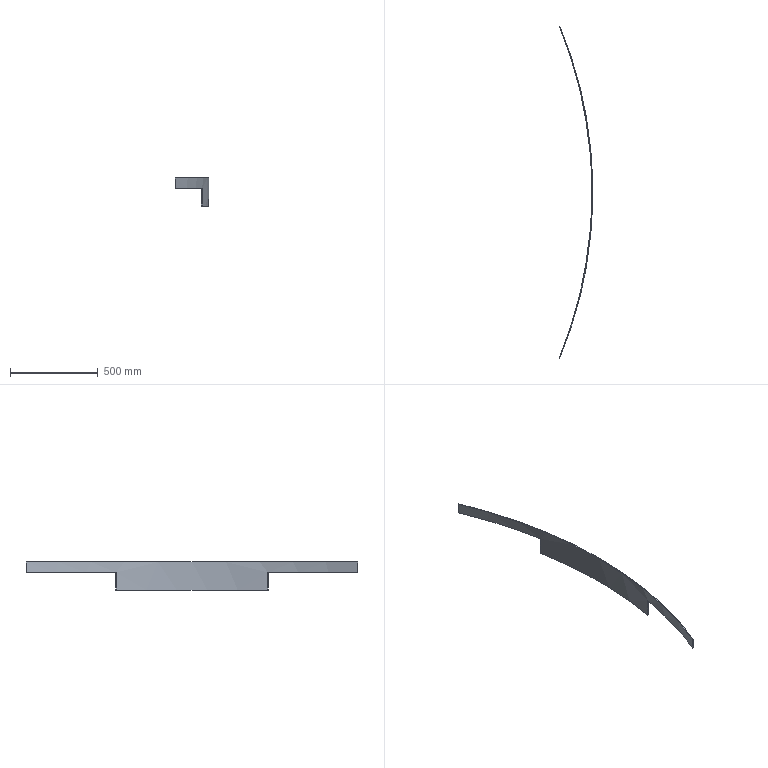Part | STEP file | 24B-Side baffle 2 | 1 solid | 10 faces | box 190.691 x 1891 x 160 mm | volume 813219 mm3 | plane 8 | cylinder 2 | commonest cylinder face diameters 4960 x1 4968 x1
STEP:
#1=CARTESIAN_POINT('',(0.,0.,0.));
#2=DIRECTION('',(0.,0.,1.));
#3=DIRECTION('',(1.,0.,0.));
#4=AXIS2_PLACEMENT_3D('',#1,#2,#3);
#5=CARTESIAN_POINT('',(2445.947,-433.125,100.));
#6=VERTEX_POINT('',#5);
#7=CARTESIAN_POINT('',(2442.009,-432.428,100.));
#8=VERTEX_POINT('',#7);
#9=CARTESIAN_POINT('',(2442.009,-432.428,100.));
#10=DIRECTION('',(-0.9847,0.1744,0.));
#11=VECTOR('',#10,1.);
#12=LINE('',#9,#11);
#13=CARTESIAN_POINT('',(0.,0.,100.));
#14=DIRECTION('',(0.,0.,1.));
#15=DIRECTION('',(1.,0.,0.));
#16=AXIS2_PLACEMENT_3D('',#13,#14,#15);
#17=PLANE('',#16);
#18=CARTESIAN_POINT('',(2442.009,-432.428));
#19=DIRECTION('',(-0.9847,0.1744));
#20=VECTOR('',#19,1.);
#21=LINE('',#18,#20);
#22=(GEOMETRIC_REPRESENTATION_CONTEXT(2)PARAMETRIC_REPRESENTATION_CONTEXT()REPRESENTATION_CONTEXT('',''));
#23=DEFINITIONAL_REPRESENTATION('',(#21),#22);
#24=PCURVE('',#17,#23);
#25=CARTESIAN_POINT('',(2442.009,-432.428,50.));
#26=DIRECTION('',(0.1744,0.9847,0.));
#27=DIRECTION('',(0.,0.,1.));
#28=AXIS2_PLACEMENT_3D('',#25,#26,#27);
#29=PLANE('',#28);
#30=CARTESIAN_POINT('',(50.,0.));
#31=DIRECTION('',(0.,-1.));
#32=VECTOR('',#31,1.);
#33=LINE('',#30,#32);
#34=(GEOMETRIC_REPRESENTATION_CONTEXT(2)PARAMETRIC_REPRESENTATION_CONTEXT()REPRESENTATION_CONTEXT('',''));
#35=DEFINITIONAL_REPRESENTATION('',(#33),#34);
#36=PCURVE('',#29,#35);
#37=SURFACE_CURVE('',#12,(#24,#36),.PCURVE_S1.);
#38=EDGE_CURVE('',#6,#8,#37,.T.);
#39=ORIENTED_EDGE('',*,*,#38,.F.);
#40=CARTESIAN_POINT('',(2297.007,-945.523,100.));
#41=VERTEX_POINT('',#40);
#42=CARTESIAN_POINT('',(0.,0.,100.));
#43=DIRECTION('',(0.,0.,-1.));
#44=DIRECTION('',(-1.,0.,0.));
#45=AXIS2_PLACEMENT_3D('',#42,#43,#44);
#46=CIRCLE('',#45,2484.);
#47=CARTESIAN_POINT('',(-2484.,0.));
#48=CARTESIAN_POINT('',(-2484.,4302.414));
#49=CARTESIAN_POINT('',(1242.,2151.207));
#50=CARTESIAN_POINT('',(4968.,0.));
#51=CARTESIAN_POINT('',(1242.,-2151.207));
#52=CARTESIAN_POINT('',(-2484.,-4302.414));
#53=CARTESIAN_POINT('',(-2484.,0.));
#54=(BOUNDED_CURVE()B_SPLINE_CURVE(2,(#47,#48,#49,#50,#51,#52,#53),.UNSPECIFIED.,.T.,.F.)B_SPLINE_CURVE_WITH_KNOTS((1,2,2,2,2,1),(-2.094,0.,2.094,4.189,6.283,8.378),.UNSPECIFIED.)CURVE()GEOMETRIC_REPRESENTATION_ITEM()RATIONAL_B_SPLINE_CURVE((1.,0.5,1.,0.5,1.,0.5,1.))REPRESENTATION_ITEM(''));
#55=(GEOMETRIC_REPRESENTATION_CONTEXT(2)PARAMETRIC_REPRESENTATION_CONTEXT()REPRESENTATION_CONTEXT('',''));
#56=DEFINITIONAL_REPRESENTATION('',(#54),#55);
#57=PCURVE('',#17,#56);
#58=CARTESIAN_POINT('',(0.,0.,2077.812));
#59=DIRECTION('',(0.,0.,-1.));
#60=DIRECTION('',(-1.,0.,0.));
#61=AXIS2_PLACEMENT_3D('',#58,#59,#60);
#62=CYLINDRICAL_SURFACE('',#61,2484.);
#63=CARTESIAN_POINT('',(0.,1977.812));
#64=DIRECTION('',(1.,0.));
#65=VECTOR('',#64,1.);
#66=LINE('',#63,#65);
#67=(GEOMETRIC_REPRESENTATION_CONTEXT(2)PARAMETRIC_REPRESENTATION_CONTEXT()REPRESENTATION_CONTEXT('',''));
#68=DEFINITIONAL_REPRESENTATION('',(#66),#67);
#69=PCURVE('',#62,#68);
#70=SURFACE_CURVE('',#46,(#57,#69),.PCURVE_S1.);
#71=EDGE_CURVE('',#6,#41,#70,.T.);
#72=ORIENTED_EDGE('',*,*,#71,.T.);
#73=CARTESIAN_POINT('',(2293.309,-944.,100.));
#74=VERTEX_POINT('',#73);
#75=CARTESIAN_POINT('',(2293.309,-944.,100.));
#76=DIRECTION('',(-0.9247,0.3806,0.));
#77=VECTOR('',#76,1.);
#78=LINE('',#75,#77);
#79=CARTESIAN_POINT('',(2293.309,-944.));
#80=DIRECTION('',(-0.9247,0.3806));
#81=VECTOR('',#80,1.);
#82=LINE('',#79,#81);
#83=(GEOMETRIC_REPRESENTATION_CONTEXT(2)PARAMETRIC_REPRESENTATION_CONTEXT()REPRESENTATION_CONTEXT('',''));
#84=DEFINITIONAL_REPRESENTATION('',(#82),#83);
#85=PCURVE('',#17,#84);
#86=CARTESIAN_POINT('',(2293.309,-944.,130.));
#87=DIRECTION('',(0.3806,0.9247,0.));
#88=DIRECTION('',(0.,0.,1.));
#89=AXIS2_PLACEMENT_3D('',#86,#87,#88);
#90=PLANE('',#89);
#91=CARTESIAN_POINT('',(-30.,0.));
#92=DIRECTION('',(0.,-1.));
#93=VECTOR('',#92,1.);
#94=LINE('',#91,#93);
#95=(GEOMETRIC_REPRESENTATION_CONTEXT(2)PARAMETRIC_REPRESENTATION_CONTEXT()REPRESENTATION_CONTEXT('',''));
#96=DEFINITIONAL_REPRESENTATION('',(#94),#95);
#97=PCURVE('',#90,#96);
#98=SURFACE_CURVE('',#78,(#85,#97),.PCURVE_S1.);
#99=EDGE_CURVE('',#41,#74,#98,.T.);
#100=ORIENTED_EDGE('',*,*,#99,.T.);
#101=CARTESIAN_POINT('',(0.,0.,100.));
#102=DIRECTION('',(0.,0.,-1.));
#103=DIRECTION('',(1.,0.,0.));
#104=AXIS2_PLACEMENT_3D('',#101,#102,#103);
#105=CIRCLE('',#104,2480.);
#106=CARTESIAN_POINT('',(2480.,0.));
#107=CARTESIAN_POINT('',(2480.,-4295.486));
#108=CARTESIAN_POINT('',(-1240.,-2147.743));
#109=CARTESIAN_POINT('',(-4960.,0.));
#110=CARTESIAN_POINT('',(-1240.,2147.743));
#111=CARTESIAN_POINT('',(2480.,4295.486));
#112=CARTESIAN_POINT('',(2480.,0.));
#113=(BOUNDED_CURVE()B_SPLINE_CURVE(2,(#106,#107,#108,#109,#110,#111,#112),.UNSPECIFIED.,.T.,.F.)B_SPLINE_CURVE_WITH_KNOTS((1,2,2,2,2,1),(-2.094,0.,2.094,4.189,6.283,8.378),.UNSPECIFIED.)CURVE()GEOMETRIC_REPRESENTATION_ITEM()RATIONAL_B_SPLINE_CURVE((1.,0.5,1.,0.5,1.,0.5,1.))REPRESENTATION_ITEM(''));
#114=(GEOMETRIC_REPRESENTATION_CONTEXT(2)PARAMETRIC_REPRESENTATION_CONTEXT()REPRESENTATION_CONTEXT('',''));
#115=DEFINITIONAL_REPRESENTATION('',(#113),#114);
#116=PCURVE('',#17,#115);
#117=CARTESIAN_POINT('',(0.,0.,2077.812));
#118=DIRECTION('',(0.,0.,-1.));
#119=DIRECTION('',(-1.,0.,0.));
#120=AXIS2_PLACEMENT_3D('',#117,#118,#119);
#121=CYLINDRICAL_SURFACE('',#120,2480.);
#122=CARTESIAN_POINT('',(3.142,1977.812));
#123=DIRECTION('',(1.,0.));
#124=VECTOR('',#123,1.);
#125=LINE('',#122,#124);
#126=(GEOMETRIC_REPRESENTATION_CONTEXT(2)PARAMETRIC_REPRESENTATION_CONTEXT()REPRESENTATION_CONTEXT('',''));
#127=DEFINITIONAL_REPRESENTATION('',(#125),#126);
#128=PCURVE('',#121,#127);
#129=SURFACE_CURVE('',#105,(#116,#128),.PCURVE_S1.);
#130=EDGE_CURVE('',#8,#74,#129,.T.);
#131=ORIENTED_EDGE('',*,*,#130,.F.);
#132=EDGE_LOOP('',(#39,#72,#100,#131));
#133=FACE_BOUND('',#132,.T.);
#134=ADVANCED_FACE('',(#133),#17,.F.);
#135=ORIENTED_EDGE('',*,*,#99,.F.);
#136=CARTESIAN_POINT('',(2297.007,-945.523,160.));
#137=VERTEX_POINT('',#136);
#138=CARTESIAN_POINT('',(2297.007,-945.523,2077.812));
#139=DIRECTION('',(0.,0.,1.));
#140=VECTOR('',#139,1.);
#141=LINE('',#138,#140);
#142=CARTESIAN_POINT('',(1947.812,4.));
#143=DIRECTION('',(1.,0.));
#144=VECTOR('',#143,1.);
#145=LINE('',#142,#144);
#146=(GEOMETRIC_REPRESENTATION_CONTEXT(2)PARAMETRIC_REPRESENTATION_CONTEXT()REPRESENTATION_CONTEXT('',''));
#147=DEFINITIONAL_REPRESENTATION('',(#145),#146);
#148=PCURVE('',#90,#147);
#149=CARTESIAN_POINT('',(3.532,0.));
#150=DIRECTION('',(0.,-1.));
#151=VECTOR('',#150,1.);
#152=LINE('',#149,#151);
#153=(GEOMETRIC_REPRESENTATION_CONTEXT(2)PARAMETRIC_REPRESENTATION_CONTEXT()REPRESENTATION_CONTEXT('',''));
#154=DEFINITIONAL_REPRESENTATION('',(#152),#153);
#155=PCURVE('',#62,#154);
#156=SURFACE_CURVE('',#141,(#148,#155),.PCURVE_S1.);
#157=EDGE_CURVE('',#41,#137,#156,.T.);
#158=ORIENTED_EDGE('',*,*,#157,.T.);
#159=CARTESIAN_POINT('',(2293.309,-944.,160.));
#160=VERTEX_POINT('',#159);
#161=CARTESIAN_POINT('',(2293.309,-944.,160.));
#162=DIRECTION('',(-0.9247,0.3806,0.));
#163=VECTOR('',#162,1.);
#164=LINE('',#161,#163);
#165=CARTESIAN_POINT('',(30.,0.));
#166=DIRECTION('',(0.,-1.));
#167=VECTOR('',#166,1.);
#168=LINE('',#165,#167);
#169=(GEOMETRIC_REPRESENTATION_CONTEXT(2)PARAMETRIC_REPRESENTATION_CONTEXT()REPRESENTATION_CONTEXT('',''));
#170=DEFINITIONAL_REPRESENTATION('',(#168),#169);
#171=PCURVE('',#90,#170);
#172=CARTESIAN_POINT('',(0.,0.,160.));
#173=DIRECTION('',(0.,0.,-1.));
#174=DIRECTION('',(-1.,0.,0.));
#175=AXIS2_PLACEMENT_3D('',#172,#173,#174);
#176=PLANE('',#175);
#177=CARTESIAN_POINT('',(-2293.309,-944.));
#178=DIRECTION('',(0.9247,0.3806));
#179=VECTOR('',#178,1.);
#180=LINE('',#177,#179);
#181=(GEOMETRIC_REPRESENTATION_CONTEXT(2)PARAMETRIC_REPRESENTATION_CONTEXT()REPRESENTATION_CONTEXT('',''));
#182=DEFINITIONAL_REPRESENTATION('',(#180),#181);
#183=PCURVE('',#176,#182);
#184=SURFACE_CURVE('',#164,(#171,#183),.PCURVE_S1.);
#185=EDGE_CURVE('',#137,#160,#184,.T.);
#186=ORIENTED_EDGE('',*,*,#185,.T.);
#187=CARTESIAN_POINT('',(2293.309,-944.,100.));
#188=DIRECTION('',(0.,0.,1.));
#189=VECTOR('',#188,1.);
#190=LINE('',#187,#189);
#191=CARTESIAN_POINT('',(-30.,0.));
#192=DIRECTION('',(1.,0.));
#193=VECTOR('',#192,1.);
#194=LINE('',#191,#193);
#195=(GEOMETRIC_REPRESENTATION_CONTEXT(2)PARAMETRIC_REPRESENTATION_CONTEXT()REPRESENTATION_CONTEXT('',''));
#196=DEFINITIONAL_REPRESENTATION('',(#194),#195);
#197=PCURVE('',#90,#196);
#198=CARTESIAN_POINT('',(3.532,1977.812));
#199=DIRECTION('',(0.,-1.));
#200=VECTOR('',#199,1.);
#201=LINE('',#198,#200);
#202=(GEOMETRIC_REPRESENTATION_CONTEXT(2)PARAMETRIC_REPRESENTATION_CONTEXT()REPRESENTATION_CONTEXT('',''));
#203=DEFINITIONAL_REPRESENTATION('',(#201),#202);
#204=PCURVE('',#121,#203);
#205=SURFACE_CURVE('',#190,(#197,#204),.PCURVE_S1.);
#206=EDGE_CURVE('',#74,#160,#205,.T.);
#207=ORIENTED_EDGE('',*,*,#206,.F.);
#208=EDGE_LOOP('',(#135,#158,#186,#207));
#209=FACE_BOUND('',#208,.T.);
#210=ADVANCED_FACE('',(#209),#90,.F.);
#211=ORIENTED_EDGE('',*,*,#185,.F.);
#212=CARTESIAN_POINT('',(2297.007,945.523,160.));
#213=VERTEX_POINT('',#212);
#214=CARTESIAN_POINT('',(0.,0.,160.));
#215=DIRECTION('',(0.,0.,1.));
#216=DIRECTION('',(-1.,0.,0.));
#217=AXIS2_PLACEMENT_3D('',#214,#215,#216);
#218=CIRCLE('',#217,2484.);
#219=CARTESIAN_POINT('',(2484.,0.));
#220=CARTESIAN_POINT('',(2484.,-4302.414));
#221=CARTESIAN_POINT('',(-1242.,-2151.207));
#222=CARTESIAN_POINT('',(-4968.,0.));
#223=CARTESIAN_POINT('',(-1242.,2151.207));
#224=CARTESIAN_POINT('',(2484.,4302.414));
#225=CARTESIAN_POINT('',(2484.,0.));
#226=(BOUNDED_CURVE()B_SPLINE_CURVE(2,(#219,#220,#221,#222,#223,#224,#225),.UNSPECIFIED.,.T.,.F.)B_SPLINE_CURVE_WITH_KNOTS((1,2,2,2,2,1),(-2.094,0.,2.094,4.189,6.283,8.378),.UNSPECIFIED.)CURVE()GEOMETRIC_REPRESENTATION_ITEM()RATIONAL_B_SPLINE_CURVE((1.,0.5,1.,0.5,1.,0.5,1.))REPRESENTATION_ITEM(''));
#227=(GEOMETRIC_REPRESENTATION_CONTEXT(2)PARAMETRIC_REPRESENTATION_CONTEXT()REPRESENTATION_CONTEXT('',''));
#228=DEFINITIONAL_REPRESENTATION('',(#226),#227);
#229=PCURVE('',#176,#228);
#230=CARTESIAN_POINT('',(6.283,1917.812));
#231=DIRECTION('',(-1.,0.));
#232=VECTOR('',#231,1.);
#233=LINE('',#230,#232);
#234=(GEOMETRIC_REPRESENTATION_CONTEXT(2)PARAMETRIC_REPRESENTATION_CONTEXT()REPRESENTATION_CONTEXT('',''));
#235=DEFINITIONAL_REPRESENTATION('',(#233),#234);
#236=PCURVE('',#62,#235);
#237=SURFACE_CURVE('',#218,(#229,#236),.PCURVE_S1.);
#238=EDGE_CURVE('',#137,#213,#237,.T.);
#239=ORIENTED_EDGE('',*,*,#238,.T.);
#240=CARTESIAN_POINT('',(2293.309,944.,160.));
#241=VERTEX_POINT('',#240);
#242=CARTESIAN_POINT('',(2293.309,944.,160.));
#243=DIRECTION('',(-0.9247,-0.3806,0.));
#244=VECTOR('',#243,1.);
#245=LINE('',#242,#244);
#246=CARTESIAN_POINT('',(-2293.309,944.));
#247=DIRECTION('',(0.9247,-0.3806));
#248=VECTOR('',#247,1.);
#249=LINE('',#246,#248);
#250=(GEOMETRIC_REPRESENTATION_CONTEXT(2)PARAMETRIC_REPRESENTATION_CONTEXT()REPRESENTATION_CONTEXT('',''));
#251=DEFINITIONAL_REPRESENTATION('',(#249),#250);
#252=PCURVE('',#176,#251);
#253=CARTESIAN_POINT('',(2293.309,944.,130.));
#254=DIRECTION('',(0.3806,-0.9247,0.));
#255=DIRECTION('',(0.,0.,-1.));
#256=AXIS2_PLACEMENT_3D('',#253,#254,#255);
#257=PLANE('',#256);
#258=CARTESIAN_POINT('',(-30.,0.));
#259=DIRECTION('',(0.,-1.));
#260=VECTOR('',#259,1.);
#261=LINE('',#258,#260);
#262=(GEOMETRIC_REPRESENTATION_CONTEXT(2)PARAMETRIC_REPRESENTATION_CONTEXT()REPRESENTATION_CONTEXT('',''));
#263=DEFINITIONAL_REPRESENTATION('',(#261),#262);
#264=PCURVE('',#257,#263);
#265=SURFACE_CURVE('',#245,(#252,#264),.PCURVE_S1.);
#266=EDGE_CURVE('',#213,#241,#265,.T.);
#267=ORIENTED_EDGE('',*,*,#266,.T.);
#268=CARTESIAN_POINT('',(0.,0.,160.));
#269=DIRECTION('',(0.,0.,1.));
#270=DIRECTION('',(1.,0.,0.));
#271=AXIS2_PLACEMENT_3D('',#268,#269,#270);
#272=CIRCLE('',#271,2480.);
#273=CARTESIAN_POINT('',(-2480.,0.));
#274=CARTESIAN_POINT('',(-2480.,4295.486));
#275=CARTESIAN_POINT('',(1240.,2147.743));
#276=CARTESIAN_POINT('',(4960.,0.));
#277=CARTESIAN_POINT('',(1240.,-2147.743));
#278=CARTESIAN_POINT('',(-2480.,-4295.486));
#279=CARTESIAN_POINT('',(-2480.,0.));
#280=(BOUNDED_CURVE()B_SPLINE_CURVE(2,(#273,#274,#275,#276,#277,#278,#279),.UNSPECIFIED.,.T.,.F.)B_SPLINE_CURVE_WITH_KNOTS((1,2,2,2,2,1),(-2.094,0.,2.094,4.189,6.283,8.378),.UNSPECIFIED.)CURVE()GEOMETRIC_REPRESENTATION_ITEM()RATIONAL_B_SPLINE_CURVE((1.,0.5,1.,0.5,1.,0.5,1.))REPRESENTATION_ITEM(''));
#281=(GEOMETRIC_REPRESENTATION_CONTEXT(2)PARAMETRIC_REPRESENTATION_CONTEXT()REPRESENTATION_CONTEXT('',''));
#282=DEFINITIONAL_REPRESENTATION('',(#280),#281);
#283=PCURVE('',#176,#282);
#284=CARTESIAN_POINT('',(9.425,1917.812));
#285=DIRECTION('',(-1.,0.));
#286=VECTOR('',#285,1.);
#287=LINE('',#284,#286);
#288=(GEOMETRIC_REPRESENTATION_CONTEXT(2)PARAMETRIC_REPRESENTATION_CONTEXT()REPRESENTATION_CONTEXT('',''));
#289=DEFINITIONAL_REPRESENTATION('',(#287),#288);
#290=PCURVE('',#121,#289);
#291=SURFACE_CURVE('',#272,(#283,#290),.PCURVE_S1.);
#292=EDGE_CURVE('',#160,#241,#291,.T.);
#293=ORIENTED_EDGE('',*,*,#292,.F.);
#294=EDGE_LOOP('',(#211,#239,#267,#293));
#295=FACE_BOUND('',#294,.T.);
#296=ADVANCED_FACE('',(#295),#176,.F.);
#297=ORIENTED_EDGE('',*,*,#266,.F.);
#298=CARTESIAN_POINT('',(2297.007,945.523,100.));
#299=VERTEX_POINT('',#298);
#300=CARTESIAN_POINT('',(2297.007,945.523,2077.812));
#301=DIRECTION('',(0.,0.,-1.));
#302=VECTOR('',#301,1.);
#303=LINE('',#300,#302);
#304=CARTESIAN_POINT('',(-1947.812,4.));
#305=DIRECTION('',(1.,0.));
#306=VECTOR('',#305,1.);
#307=LINE('',#304,#306);
#308=(GEOMETRIC_REPRESENTATION_CONTEXT(2)PARAMETRIC_REPRESENTATION_CONTEXT()REPRESENTATION_CONTEXT('',''));
#309=DEFINITIONAL_REPRESENTATION('',(#307),#308);
#310=PCURVE('',#257,#309);
#311=CARTESIAN_POINT('',(2.751,0.));
#312=DIRECTION('',(0.,1.));
#313=VECTOR('',#312,1.);
#314=LINE('',#311,#313);
#315=(GEOMETRIC_REPRESENTATION_CONTEXT(2)PARAMETRIC_REPRESENTATION_CONTEXT()REPRESENTATION_CONTEXT('',''));
#316=DEFINITIONAL_REPRESENTATION('',(#314),#315);
#317=PCURVE('',#62,#316);
#318=SURFACE_CURVE('',#303,(#310,#317),.PCURVE_S1.);
#319=EDGE_CURVE('',#213,#299,#318,.T.);
#320=ORIENTED_EDGE('',*,*,#319,.T.);
#321=CARTESIAN_POINT('',(2293.309,944.,100.));
#322=VERTEX_POINT('',#321);
#323=CARTESIAN_POINT('',(2293.309,944.,100.));
#324=DIRECTION('',(-0.9247,-0.3806,0.));
#325=VECTOR('',#324,1.);
#326=LINE('',#323,#325);
#327=CARTESIAN_POINT('',(30.,0.));
#328=DIRECTION('',(0.,-1.));
#329=VECTOR('',#328,1.);
#330=LINE('',#327,#329);
#331=(GEOMETRIC_REPRESENTATION_CONTEXT(2)PARAMETRIC_REPRESENTATION_CONTEXT()REPRESENTATION_CONTEXT('',''));
#332=DEFINITIONAL_REPRESENTATION('',(#330),#331);
#333=PCURVE('',#257,#332);
#334=CARTESIAN_POINT('',(0.,0.,100.));
#335=DIRECTION('',(0.,0.,1.));
#336=DIRECTION('',(1.,0.,0.));
#337=AXIS2_PLACEMENT_3D('',#334,#335,#336);
#338=PLANE('',#337);
#339=CARTESIAN_POINT('',(2293.309,944.));
#340=DIRECTION('',(-0.9247,-0.3806));
#341=VECTOR('',#340,1.);
#342=LINE('',#339,#341);
#343=(GEOMETRIC_REPRESENTATION_CONTEXT(2)PARAMETRIC_REPRESENTATION_CONTEXT()REPRESENTATION_CONTEXT('',''));
#344=DEFINITIONAL_REPRESENTATION('',(#342),#343);
#345=PCURVE('',#338,#344);
#346=SURFACE_CURVE('',#326,(#333,#345),.PCURVE_S1.);
#347=EDGE_CURVE('',#299,#322,#346,.T.);
#348=ORIENTED_EDGE('',*,*,#347,.T.);
#349=CARTESIAN_POINT('',(2293.309,944.,160.));
#350=DIRECTION('',(0.,0.,-1.));
#351=VECTOR('',#350,1.);
#352=LINE('',#349,#351);
#353=CARTESIAN_POINT('',(-30.,0.));
#354=DIRECTION('',(1.,0.));
#355=VECTOR('',#354,1.);
#356=LINE('',#353,#355);
#357=(GEOMETRIC_REPRESENTATION_CONTEXT(2)PARAMETRIC_REPRESENTATION_CONTEXT()REPRESENTATION_CONTEXT('',''));
#358=DEFINITIONAL_REPRESENTATION('',(#356),#357);
#359=PCURVE('',#257,#358);
#360=CARTESIAN_POINT('',(2.751,1917.812));
#361=DIRECTION('',(0.,1.));
#362=VECTOR('',#361,1.);
#363=LINE('',#360,#362);
#364=(GEOMETRIC_REPRESENTATION_CONTEXT(2)PARAMETRIC_REPRESENTATION_CONTEXT()REPRESENTATION_CONTEXT('',''));
#365=DEFINITIONAL_REPRESENTATION('',(#363),#364);
#366=PCURVE('',#121,#365);
#367=SURFACE_CURVE('',#352,(#359,#366),.PCURVE_S1.);
#368=EDGE_CURVE('',#241,#322,#367,.T.);
#369=ORIENTED_EDGE('',*,*,#368,.F.);
#370=EDGE_LOOP('',(#297,#320,#348,#369));
#371=FACE_BOUND('',#370,.T.);
#372=ADVANCED_FACE('',(#371),#257,.F.);
#373=ORIENTED_EDGE('',*,*,#347,.F.);
#374=CARTESIAN_POINT('',(2445.947,433.125,100.));
#375=VERTEX_POINT('',#374);
#376=CARTESIAN_POINT('',(0.,0.,100.));
#377=DIRECTION('',(0.,0.,-1.));
#378=DIRECTION('',(-1.,0.,0.));
#379=AXIS2_PLACEMENT_3D('',#376,#377,#378);
#380=CIRCLE('',#379,2484.);
#381=CARTESIAN_POINT('',(-2484.,0.));
#382=CARTESIAN_POINT('',(-2484.,4302.414));
#383=CARTESIAN_POINT('',(1242.,2151.207));
#384=CARTESIAN_POINT('',(4968.,0.));
#385=CARTESIAN_POINT('',(1242.,-2151.207));
#386=CARTESIAN_POINT('',(-2484.,-4302.414));
#387=CARTESIAN_POINT('',(-2484.,0.));
#388=(BOUNDED_CURVE()B_SPLINE_CURVE(2,(#381,#382,#383,#384,#385,#386,#387),.UNSPECIFIED.,.T.,.F.)B_SPLINE_CURVE_WITH_KNOTS((1,2,2,2,2,1),(-2.094,0.,2.094,4.189,6.283,8.378),.UNSPECIFIED.)CURVE()GEOMETRIC_REPRESENTATION_ITEM()RATIONAL_B_SPLINE_CURVE((1.,0.5,1.,0.5,1.,0.5,1.))REPRESENTATION_ITEM(''));
#389=(GEOMETRIC_REPRESENTATION_CONTEXT(2)PARAMETRIC_REPRESENTATION_CONTEXT()REPRESENTATION_CONTEXT('',''));
#390=DEFINITIONAL_REPRESENTATION('',(#388),#389);
#391=PCURVE('',#338,#390);
#392=CARTESIAN_POINT('',(0.,1977.812));
#393=DIRECTION('',(1.,0.));
#394=VECTOR('',#393,1.);
#395=LINE('',#392,#394);
#396=(GEOMETRIC_REPRESENTATION_CONTEXT(2)PARAMETRIC_REPRESENTATION_CONTEXT()REPRESENTATION_CONTEXT('',''));
#397=DEFINITIONAL_REPRESENTATION('',(#395),#396);
#398=PCURVE('',#62,#397);
#399=SURFACE_CURVE('',#380,(#391,#398),.PCURVE_S1.);
#400=EDGE_CURVE('',#299,#375,#399,.T.);
#401=ORIENTED_EDGE('',*,*,#400,.T.);
#402=CARTESIAN_POINT('',(2442.009,432.428,100.));
#403=VERTEX_POINT('',#402);
#404=CARTESIAN_POINT('',(2442.009,432.428,100.));
#405=DIRECTION('',(-0.9847,-0.1744,0.));
#406=VECTOR('',#405,1.);
#407=LINE('',#404,#406);
#408=CARTESIAN_POINT('',(2442.009,432.428));
#409=DIRECTION('',(-0.9847,-0.1744));
#410=VECTOR('',#409,1.);
#411=LINE('',#408,#410);
#412=(GEOMETRIC_REPRESENTATION_CONTEXT(2)PARAMETRIC_REPRESENTATION_CONTEXT()REPRESENTATION_CONTEXT('',''));
#413=DEFINITIONAL_REPRESENTATION('',(#411),#412);
#414=PCURVE('',#338,#413);
#415=CARTESIAN_POINT('',(2442.009,432.428,50.));
#416=DIRECTION('',(0.1744,-0.9847,0.));
#417=DIRECTION('',(0.,0.,-1.));
#418=AXIS2_PLACEMENT_3D('',#415,#416,#417);
#419=PLANE('',#418);
#420=CARTESIAN_POINT('',(-50.,0.));
#421=DIRECTION('',(0.,-1.));
#422=VECTOR('',#421,1.);
#423=LINE('',#420,#422);
#424=(GEOMETRIC_REPRESENTATION_CONTEXT(2)PARAMETRIC_REPRESENTATION_CONTEXT()REPRESENTATION_CONTEXT('',''));
#425=DEFINITIONAL_REPRESENTATION('',(#423),#424);
#426=PCURVE('',#419,#425);
#427=SURFACE_CURVE('',#407,(#414,#426),.PCURVE_S1.);
#428=EDGE_CURVE('',#375,#403,#427,.T.);
#429=ORIENTED_EDGE('',*,*,#428,.T.);
#430=CARTESIAN_POINT('',(0.,0.,100.));
#431=DIRECTION('',(0.,0.,-1.));
#432=DIRECTION('',(1.,0.,0.));
#433=AXIS2_PLACEMENT_3D('',#430,#431,#432);
#434=CIRCLE('',#433,2480.);
#435=CARTESIAN_POINT('',(2480.,0.));
#436=CARTESIAN_POINT('',(2480.,-4295.486));
#437=CARTESIAN_POINT('',(-1240.,-2147.743));
#438=CARTESIAN_POINT('',(-4960.,0.));
#439=CARTESIAN_POINT('',(-1240.,2147.743));
#440=CARTESIAN_POINT('',(2480.,4295.486));
#441=CARTESIAN_POINT('',(2480.,0.));
#442=(BOUNDED_CURVE()B_SPLINE_CURVE(2,(#435,#436,#437,#438,#439,#440,#441),.UNSPECIFIED.,.T.,.F.)B_SPLINE_CURVE_WITH_KNOTS((1,2,2,2,2,1),(-2.094,0.,2.094,4.189,6.283,8.378),.UNSPECIFIED.)CURVE()GEOMETRIC_REPRESENTATION_ITEM()RATIONAL_B_SPLINE_CURVE((1.,0.5,1.,0.5,1.,0.5,1.))REPRESENTATION_ITEM(''));
#443=(GEOMETRIC_REPRESENTATION_CONTEXT(2)PARAMETRIC_REPRESENTATION_CONTEXT()REPRESENTATION_CONTEXT('',''));
#444=DEFINITIONAL_REPRESENTATION('',(#442),#443);
#445=PCURVE('',#338,#444);
#446=CARTESIAN_POINT('',(-3.142,1977.812));
#447=DIRECTION('',(1.,0.));
#448=VECTOR('',#447,1.);
#449=LINE('',#446,#448);
#450=(GEOMETRIC_REPRESENTATION_CONTEXT(2)PARAMETRIC_REPRESENTATION_CONTEXT()REPRESENTATION_CONTEXT('',''));
#451=DEFINITIONAL_REPRESENTATION('',(#449),#450);
#452=PCURVE('',#121,#451);
#453=SURFACE_CURVE('',#434,(#445,#452),.PCURVE_S1.);
#454=EDGE_CURVE('',#322,#403,#453,.T.);
#455=ORIENTED_EDGE('',*,*,#454,.F.);
#456=EDGE_LOOP('',(#373,#401,#429,#455));
#457=FACE_BOUND('',#456,.T.);
#458=ADVANCED_FACE('',(#457),#338,.F.);
#459=ORIENTED_EDGE('',*,*,#428,.F.);
#460=CARTESIAN_POINT('',(2445.947,433.125,0.));
#461=VERTEX_POINT('',#460);
#462=CARTESIAN_POINT('',(2445.947,433.125,2077.812));
#463=DIRECTION('',(0.,0.,-1.));
#464=VECTOR('',#463,1.);
#465=LINE('',#462,#464);
#466=CARTESIAN_POINT('',(-2027.812,4.));
#467=DIRECTION('',(1.,0.));
#468=VECTOR('',#467,1.);
#469=LINE('',#466,#468);
#470=(GEOMETRIC_REPRESENTATION_CONTEXT(2)PARAMETRIC_REPRESENTATION_CONTEXT()REPRESENTATION_CONTEXT('',''));
#471=DEFINITIONAL_REPRESENTATION('',(#469),#470);
#472=PCURVE('',#419,#471);
#473=CARTESIAN_POINT('',(2.966,0.));
#474=DIRECTION('',(0.,1.));
#475=VECTOR('',#474,1.);
#476=LINE('',#473,#475);
#477=(GEOMETRIC_REPRESENTATION_CONTEXT(2)PARAMETRIC_REPRESENTATION_CONTEXT()REPRESENTATION_CONTEXT('',''));
#478=DEFINITIONAL_REPRESENTATION('',(#476),#477);
#479=PCURVE('',#62,#478);
#480=SURFACE_CURVE('',#465,(#472,#479),.PCURVE_S1.);
#481=EDGE_CURVE('',#375,#461,#480,.T.);
#482=ORIENTED_EDGE('',*,*,#481,.T.);
#483=CARTESIAN_POINT('',(2442.009,432.428,0.));
#484=VERTEX_POINT('',#483);
#485=CARTESIAN_POINT('',(2442.009,432.428,0.));
#486=DIRECTION('',(-0.9847,-0.1744,0.));
#487=VECTOR('',#486,1.);
#488=LINE('',#485,#487);
#489=CARTESIAN_POINT('',(50.,0.));
#490=DIRECTION('',(0.,-1.));
#491=VECTOR('',#490,1.);
#492=LINE('',#489,#491);
#493=(GEOMETRIC_REPRESENTATION_CONTEXT(2)PARAMETRIC_REPRESENTATION_CONTEXT()REPRESENTATION_CONTEXT('',''));
#494=DEFINITIONAL_REPRESENTATION('',(#492),#493);
#495=PCURVE('',#419,#494);
#496=CARTESIAN_POINT('',(0.,0.,0.));
#497=DIRECTION('',(0.,0.,1.));
#498=DIRECTION('',(1.,0.,0.));
#499=AXIS2_PLACEMENT_3D('',#496,#497,#498);
#500=PLANE('',#499);
#501=CARTESIAN_POINT('',(2442.009,432.428));
#502=DIRECTION('',(-0.9847,-0.1744));
#503=VECTOR('',#502,1.);
#504=LINE('',#501,#503);
#505=(GEOMETRIC_REPRESENTATION_CONTEXT(2)PARAMETRIC_REPRESENTATION_CONTEXT()REPRESENTATION_CONTEXT('',''));
#506=DEFINITIONAL_REPRESENTATION('',(#504),#505);
#507=PCURVE('',#500,#506);
#508=SURFACE_CURVE('',#488,(#495,#507),.PCURVE_S1.);
#509=EDGE_CURVE('',#461,#484,#508,.T.);
#510=ORIENTED_EDGE('',*,*,#509,.T.);
#511=CARTESIAN_POINT('',(2442.009,432.428,0.));
#512=DIRECTION('',(0.,0.,-1.));
#513=VECTOR('',#512,1.);
#514=LINE('',#511,#513);
#515=CARTESIAN_POINT('',(50.,0.));
#516=DIRECTION('',(1.,0.));
#517=VECTOR('',#516,1.);
#518=LINE('',#515,#517);
#519=(GEOMETRIC_REPRESENTATION_CONTEXT(2)PARAMETRIC_REPRESENTATION_CONTEXT()REPRESENTATION_CONTEXT('',''));
#520=DEFINITIONAL_REPRESENTATION('',(#518),#519);
#521=PCURVE('',#419,#520);
#522=CARTESIAN_POINT('',(2.966,2077.812));
#523=DIRECTION('',(0.,1.));
#524=VECTOR('',#523,1.);
#525=LINE('',#522,#524);
#526=(GEOMETRIC_REPRESENTATION_CONTEXT(2)PARAMETRIC_REPRESENTATION_CONTEXT()REPRESENTATION_CONTEXT('',''));
#527=DEFINITIONAL_REPRESENTATION('',(#525),#526);
#528=PCURVE('',#121,#527);
#529=SURFACE_CURVE('',#514,(#521,#528),.PCURVE_S1.);
#530=EDGE_CURVE('',#403,#484,#529,.T.);
#531=ORIENTED_EDGE('',*,*,#530,.F.);
#532=EDGE_LOOP('',(#459,#482,#510,#531));
#533=FACE_BOUND('',#532,.T.);
#534=ADVANCED_FACE('',(#533),#419,.F.);
#535=ORIENTED_EDGE('',*,*,#509,.F.);
#536=CARTESIAN_POINT('',(2445.947,-433.125,0.));
#537=VERTEX_POINT('',#536);
#538=CARTESIAN_POINT('',(0.,0.,0.));
#539=DIRECTION('',(0.,0.,-1.));
#540=DIRECTION('',(-1.,0.,0.));
#541=AXIS2_PLACEMENT_3D('',#538,#539,#540);
#542=CIRCLE('',#541,2484.);
#543=CARTESIAN_POINT('',(-2484.,0.));
#544=CARTESIAN_POINT('',(-2484.,4302.414));
#545=CARTESIAN_POINT('',(1242.,2151.207));
#546=CARTESIAN_POINT('',(4968.,0.));
#547=CARTESIAN_POINT('',(1242.,-2151.207));
#548=CARTESIAN_POINT('',(-2484.,-4302.414));
#549=CARTESIAN_POINT('',(-2484.,0.));
#550=(BOUNDED_CURVE()B_SPLINE_CURVE(2,(#543,#544,#545,#546,#547,#548,#549),.UNSPECIFIED.,.T.,.F.)B_SPLINE_CURVE_WITH_KNOTS((1,2,2,2,2,1),(-2.094,0.,2.094,4.189,6.283,8.378),.UNSPECIFIED.)CURVE()GEOMETRIC_REPRESENTATION_ITEM()RATIONAL_B_SPLINE_CURVE((1.,0.5,1.,0.5,1.,0.5,1.))REPRESENTATION_ITEM(''));
#551=(GEOMETRIC_REPRESENTATION_CONTEXT(2)PARAMETRIC_REPRESENTATION_CONTEXT()REPRESENTATION_CONTEXT('',''));
#552=DEFINITIONAL_REPRESENTATION('',(#550),#551);
#553=PCURVE('',#500,#552);
#554=CARTESIAN_POINT('',(0.,2077.812));
#555=DIRECTION('',(1.,0.));
#556=VECTOR('',#555,1.);
#557=LINE('',#554,#556);
#558=(GEOMETRIC_REPRESENTATION_CONTEXT(2)PARAMETRIC_REPRESENTATION_CONTEXT()REPRESENTATION_CONTEXT('',''));
#559=DEFINITIONAL_REPRESENTATION('',(#557),#558);
#560=PCURVE('',#62,#559);
#561=SURFACE_CURVE('',#542,(#553,#560),.PCURVE_S1.);
#562=EDGE_CURVE('',#461,#537,#561,.T.);
#563=ORIENTED_EDGE('',*,*,#562,.T.);
#564=CARTESIAN_POINT('',(2442.009,-432.428,0.));
#565=VERTEX_POINT('',#564);
#566=CARTESIAN_POINT('',(2442.009,-432.428,0.));
#567=DIRECTION('',(-0.9847,0.1744,0.));
#568=VECTOR('',#567,1.);
#569=LINE('',#566,#568);
#570=CARTESIAN_POINT('',(2442.009,-432.428));
#571=DIRECTION('',(-0.9847,0.1744));
#572=VECTOR('',#571,1.);
#573=LINE('',#570,#572);
#574=(GEOMETRIC_REPRESENTATION_CONTEXT(2)PARAMETRIC_REPRESENTATION_CONTEXT()REPRESENTATION_CONTEXT('',''));
#575=DEFINITIONAL_REPRESENTATION('',(#573),#574);
#576=PCURVE('',#500,#575);
#577=CARTESIAN_POINT('',(-50.,0.));
#578=DIRECTION('',(0.,-1.));
#579=VECTOR('',#578,1.);
#580=LINE('',#577,#579);
#581=(GEOMETRIC_REPRESENTATION_CONTEXT(2)PARAMETRIC_REPRESENTATION_CONTEXT()REPRESENTATION_CONTEXT('',''));
#582=DEFINITIONAL_REPRESENTATION('',(#580),#581);
#583=PCURVE('',#29,#582);
#584=SURFACE_CURVE('',#569,(#576,#583),.PCURVE_S1.);
#585=EDGE_CURVE('',#537,#565,#584,.T.);
#586=ORIENTED_EDGE('',*,*,#585,.T.);
#587=CARTESIAN_POINT('',(0.,0.,0.));
#588=DIRECTION('',(0.,0.,-1.));
#589=DIRECTION('',(-1.,0.,0.));
#590=AXIS2_PLACEMENT_3D('',#587,#588,#589);
#591=CIRCLE('',#590,2480.);
#592=CARTESIAN_POINT('',(-2480.,0.));
#593=CARTESIAN_POINT('',(-2480.,4295.486));
#594=CARTESIAN_POINT('',(1240.,2147.743));
#595=CARTESIAN_POINT('',(4960.,0.));
#596=CARTESIAN_POINT('',(1240.,-2147.743));
#597=CARTESIAN_POINT('',(-2480.,-4295.486));
#598=CARTESIAN_POINT('',(-2480.,0.));
#599=(BOUNDED_CURVE()B_SPLINE_CURVE(2,(#592,#593,#594,#595,#596,#597,#598),.UNSPECIFIED.,.T.,.F.)B_SPLINE_CURVE_WITH_KNOTS((1,2,2,2,2,1),(-2.094,0.,2.094,4.189,6.283,8.378),.UNSPECIFIED.)CURVE()GEOMETRIC_REPRESENTATION_ITEM()RATIONAL_B_SPLINE_CURVE((1.,0.5,1.,0.5,1.,0.5,1.))REPRESENTATION_ITEM(''));
#600=(GEOMETRIC_REPRESENTATION_CONTEXT(2)PARAMETRIC_REPRESENTATION_CONTEXT()REPRESENTATION_CONTEXT('',''));
#601=DEFINITIONAL_REPRESENTATION('',(#599),#600);
#602=PCURVE('',#500,#601);
#603=CARTESIAN_POINT('',(0.,2077.812));
#604=DIRECTION('',(1.,0.));
#605=VECTOR('',#604,1.);
#606=LINE('',#603,#605);
#607=(GEOMETRIC_REPRESENTATION_CONTEXT(2)PARAMETRIC_REPRESENTATION_CONTEXT()REPRESENTATION_CONTEXT('',''));
#608=DEFINITIONAL_REPRESENTATION('',(#606),#607);
#609=PCURVE('',#121,#608);
#610=SURFACE_CURVE('',#591,(#602,#609),.PCURVE_S1.);
#611=EDGE_CURVE('',#484,#565,#610,.T.);
#612=ORIENTED_EDGE('',*,*,#611,.F.);
#613=EDGE_LOOP('',(#535,#563,#586,#612));
#614=FACE_BOUND('',#613,.T.);
#615=ADVANCED_FACE('',(#614),#500,.F.);
#616=CARTESIAN_POINT('',(2445.947,-433.125,2077.812));
#617=DIRECTION('',(0.,0.,1.));
#618=VECTOR('',#617,1.);
#619=LINE('',#616,#618);
#620=CARTESIAN_POINT('',(2027.812,4.));
#621=DIRECTION('',(1.,0.));
#622=VECTOR('',#621,1.);
#623=LINE('',#620,#622);
#624=(GEOMETRIC_REPRESENTATION_CONTEXT(2)PARAMETRIC_REPRESENTATION_CONTEXT()REPRESENTATION_CONTEXT('',''));
#625=DEFINITIONAL_REPRESENTATION('',(#623),#624);
#626=PCURVE('',#29,#625);
#627=CARTESIAN_POINT('',(3.317,0.));
#628=DIRECTION('',(0.,-1.));
#629=VECTOR('',#628,1.);
#630=LINE('',#627,#629);
#631=(GEOMETRIC_REPRESENTATION_CONTEXT(2)PARAMETRIC_REPRESENTATION_CONTEXT()REPRESENTATION_CONTEXT('',''));
#632=DEFINITIONAL_REPRESENTATION('',(#630),#631);
#633=PCURVE('',#62,#632);
#634=SURFACE_CURVE('',#619,(#626,#633),.PCURVE_S1.);
#635=EDGE_CURVE('',#537,#6,#634,.T.);
#636=ORIENTED_EDGE('',*,*,#635,.T.);
#637=ORIENTED_EDGE('',*,*,#38,.T.);
#638=CARTESIAN_POINT('',(2442.009,-432.428,100.));
#639=DIRECTION('',(0.,0.,1.));
#640=VECTOR('',#639,1.);
#641=LINE('',#638,#640);
#642=CARTESIAN_POINT('',(50.,0.));
#643=DIRECTION('',(1.,0.));
#644=VECTOR('',#643,1.);
#645=LINE('',#642,#644);
#646=(GEOMETRIC_REPRESENTATION_CONTEXT(2)PARAMETRIC_REPRESENTATION_CONTEXT()REPRESENTATION_CONTEXT('',''));
#647=DEFINITIONAL_REPRESENTATION('',(#645),#646);
#648=PCURVE('',#29,#647);
#649=CARTESIAN_POINT('',(3.317,1977.812));
#650=DIRECTION('',(0.,-1.));
#651=VECTOR('',#650,1.);
#652=LINE('',#649,#651);
#653=(GEOMETRIC_REPRESENTATION_CONTEXT(2)PARAMETRIC_REPRESENTATION_CONTEXT()REPRESENTATION_CONTEXT('',''));
#654=DEFINITIONAL_REPRESENTATION('',(#652),#653);
#655=PCURVE('',#121,#654);
#656=SURFACE_CURVE('',#641,(#648,#655),.PCURVE_S1.);
#657=EDGE_CURVE('',#565,#8,#656,.T.);
#658=ORIENTED_EDGE('',*,*,#657,.F.);
#659=ORIENTED_EDGE('',*,*,#585,.F.);
#660=EDGE_LOOP('',(#636,#637,#658,#659));
#661=FACE_BOUND('',#660,.T.);
#662=ADVANCED_FACE('',(#661),#29,.F.);
#663=ORIENTED_EDGE('',*,*,#530,.F.);
#664=ORIENTED_EDGE('',*,*,#454,.F.);
#665=ORIENTED_EDGE('',*,*,#368,.F.);
#666=ORIENTED_EDGE('',*,*,#292,.F.);
#667=ORIENTED_EDGE('',*,*,#206,.F.);
#668=ORIENTED_EDGE('',*,*,#130,.F.);
#669=ORIENTED_EDGE('',*,*,#657,.F.);
#670=ORIENTED_EDGE('',*,*,#611,.F.);
#671=EDGE_LOOP('',(#663,#664,#665,#666,#667,#668,#669,#670));
#672=FACE_BOUND('',#671,.F.);
#673=ADVANCED_FACE('',(#672),#121,.F.);
#674=ORIENTED_EDGE('',*,*,#562,.F.);
#675=ORIENTED_EDGE('',*,*,#481,.F.);
#676=ORIENTED_EDGE('',*,*,#400,.F.);
#677=ORIENTED_EDGE('',*,*,#319,.F.);
#678=ORIENTED_EDGE('',*,*,#238,.F.);
#679=ORIENTED_EDGE('',*,*,#157,.F.);
#680=ORIENTED_EDGE('',*,*,#71,.F.);
#681=ORIENTED_EDGE('',*,*,#635,.F.);
#682=EDGE_LOOP('',(#674,#675,#676,#677,#678,#679,#680,#681));
#683=FACE_BOUND('',#682,.T.);
#684=ADVANCED_FACE('',(#683),#62,.T.);
#685=CLOSED_SHELL('',(#134,#210,#296,#372,#458,#534,#615,#662,#673,#684));
#686=MANIFOLD_SOLID_BREP('',#685);
#687=(LENGTH_UNIT()NAMED_UNIT(*)SI_UNIT(.MILLI.,.METRE.));
#688=UNCERTAINTY_MEASURE_WITH_UNIT(LENGTH_MEASURE(0.0000001),#687,'','');
#689=(NAMED_UNIT(*)PLANE_ANGLE_UNIT()SI_UNIT($,.RADIAN.));
#690=(NAMED_UNIT(*)SI_UNIT($,.STERADIAN.)SOLID_ANGLE_UNIT());
#691=(GEOMETRIC_REPRESENTATION_CONTEXT(3)GLOBAL_UNCERTAINTY_ASSIGNED_CONTEXT((#688))GLOBAL_UNIT_ASSIGNED_CONTEXT((#687,#689,#690))REPRESENTATION_CONTEXT('',''));
#692=ADVANCED_BREP_SHAPE_REPRESENTATION('',(#4,#686),#691);